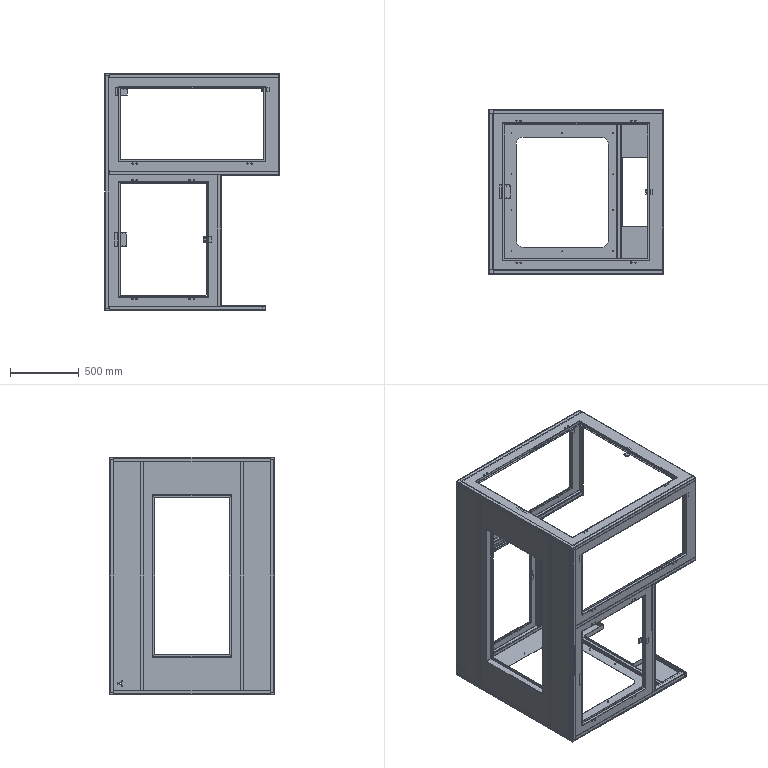Part | SolidWorks | features EdgeFlange 19, ICE 17, FlatPattern 11, HoleWzd 11, Fillet 7, SMBaseFlange 7, SheetMetal 7, MirrorSolid 2, 3DProfileFeature 1, Cut 1, MirrorPattern 1, WeldMemberFeat 1, WeldmentFeature 1 | 26 solids | 1525 faces | box 1270 x 1200 x 1725 mm | volume 14201565 mm3 | plane 925 | cylinder 488 | spline 112 | commonest cylinder face diameters 0.6 x86 4.6 x86 5 x84 4 x60 8 x60 7 x44